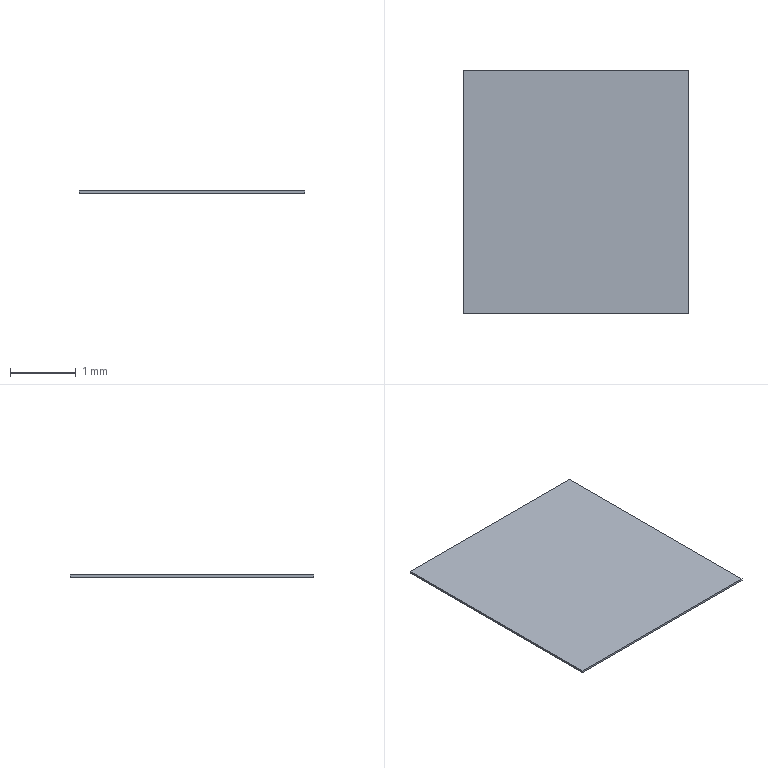Part | Creo | 1 solid | 6 faces | box 3.43 x 3.71 x 0.03048 mm | volume 0.3879 mm3 | plane 6
STEP:
#1=CARTESIAN_POINT('',(0.,0.,0.));
#2=DIRECTION('',(0.,0.,1.));
#3=DIRECTION('',(1.,0.,0.));
#4=AXIS2_PLACEMENT_3D('',#1,#2,#3);
#5=CARTESIAN_POINT('',(-1.775,-1.855,0.));
#6=VERTEX_POINT('',#5);
#7=CARTESIAN_POINT('',(1.655,-1.855,0.));
#8=VERTEX_POINT('',#7);
#9=CARTESIAN_POINT('',(-1.775,-1.855,0.));
#10=DIRECTION('',(1.,0.,0.));
#11=VECTOR('',#10,3.43);
#12=LINE('',#9,#11);
#13=EDGE_CURVE('',#6,#8,#12,.T.);
#14=ORIENTED_EDGE('',*,*,#13,.T.);
#15=CARTESIAN_POINT('',(1.655,1.855,0.));
#16=VERTEX_POINT('',#15);
#17=CARTESIAN_POINT('',(1.655,-1.855,0.));
#18=DIRECTION('',(0.,1.,0.));
#19=VECTOR('',#18,3.71);
#20=LINE('',#17,#19);
#21=EDGE_CURVE('',#8,#16,#20,.T.);
#22=ORIENTED_EDGE('',*,*,#21,.T.);
#23=CARTESIAN_POINT('',(-1.775,1.855,0.));
#24=VERTEX_POINT('',#23);
#25=CARTESIAN_POINT('',(1.655,1.855,0.));
#26=DIRECTION('',(-1.,0.,0.));
#27=VECTOR('',#26,3.43);
#28=LINE('',#25,#27);
#29=EDGE_CURVE('',#16,#24,#28,.T.);
#30=ORIENTED_EDGE('',*,*,#29,.T.);
#31=CARTESIAN_POINT('',(-1.775,1.855,0.));
#32=DIRECTION('',(0.,-1.,0.));
#33=VECTOR('',#32,3.71);
#34=LINE('',#31,#33);
#35=EDGE_CURVE('',#24,#6,#34,.T.);
#36=ORIENTED_EDGE('',*,*,#35,.T.);
#37=EDGE_LOOP('',(#14,#22,#30,#36));
#38=FACE_OUTER_BOUND('',#37,.F.);
#39=CARTESIAN_POINT('',(0.,0.,0.));
#40=DIRECTION('',(0.,0.,1.));
#41=DIRECTION('',(1.,0.,0.));
#42=AXIS2_PLACEMENT_3D('',#39,#40,#41);
#43=PLANE('',#42);
#44=ADVANCED_FACE('',(#38),#43,.F.);
#45=ORIENTED_EDGE('',*,*,#13,.F.);
#46=CARTESIAN_POINT('',(-1.775,-1.855,0.03048));
#47=VERTEX_POINT('',#46);
#48=CARTESIAN_POINT('',(-1.775,-1.855,0.));
#49=DIRECTION('',(0.,0.,1.));
#50=VECTOR('',#49,0.03048);
#51=LINE('',#48,#50);
#52=EDGE_CURVE('',#6,#47,#51,.T.);
#53=ORIENTED_EDGE('',*,*,#52,.T.);
#54=CARTESIAN_POINT('',(1.655,-1.855,0.03048));
#55=VERTEX_POINT('',#54);
#56=CARTESIAN_POINT('',(-1.775,-1.855,0.03048));
#57=DIRECTION('',(1.,0.,0.));
#58=VECTOR('',#57,3.43);
#59=LINE('',#56,#58);
#60=EDGE_CURVE('',#47,#55,#59,.T.);
#61=ORIENTED_EDGE('',*,*,#60,.T.);
#62=CARTESIAN_POINT('',(1.655,-1.855,0.));
#63=DIRECTION('',(0.,0.,1.));
#64=VECTOR('',#63,0.03048);
#65=LINE('',#62,#64);
#66=EDGE_CURVE('',#8,#55,#65,.T.);
#67=ORIENTED_EDGE('',*,*,#66,.F.);
#68=EDGE_LOOP('',(#45,#53,#61,#67));
#69=FACE_OUTER_BOUND('',#68,.F.);
#70=CARTESIAN_POINT('',(-1.775,-1.855,0.));
#71=DIRECTION('',(0.,-1.,0.));
#72=DIRECTION('',(1.,0.,0.));
#73=AXIS2_PLACEMENT_3D('',#70,#71,#72);
#74=PLANE('',#73);
#75=ADVANCED_FACE('',(#69),#74,.T.);
#76=ORIENTED_EDGE('',*,*,#35,.F.);
#77=CARTESIAN_POINT('',(-1.775,1.855,0.03048));
#78=VERTEX_POINT('',#77);
#79=CARTESIAN_POINT('',(-1.775,1.855,0.));
#80=DIRECTION('',(0.,0.,1.));
#81=VECTOR('',#80,0.03048);
#82=LINE('',#79,#81);
#83=EDGE_CURVE('',#24,#78,#82,.T.);
#84=ORIENTED_EDGE('',*,*,#83,.T.);
#85=CARTESIAN_POINT('',(-1.775,1.855,0.03048));
#86=DIRECTION('',(0.,-1.,0.));
#87=VECTOR('',#86,3.71);
#88=LINE('',#85,#87);
#89=EDGE_CURVE('',#78,#47,#88,.T.);
#90=ORIENTED_EDGE('',*,*,#89,.T.);
#91=ORIENTED_EDGE('',*,*,#52,.F.);
#92=EDGE_LOOP('',(#76,#84,#90,#91));
#93=FACE_OUTER_BOUND('',#92,.F.);
#94=CARTESIAN_POINT('',(-1.775,1.855,0.));
#95=DIRECTION('',(-1.,0.,0.));
#96=DIRECTION('',(0.,-1.,0.));
#97=AXIS2_PLACEMENT_3D('',#94,#95,#96);
#98=PLANE('',#97);
#99=ADVANCED_FACE('',(#93),#98,.T.);
#100=ORIENTED_EDGE('',*,*,#29,.F.);
#101=CARTESIAN_POINT('',(1.655,1.855,0.03048));
#102=VERTEX_POINT('',#101);
#103=CARTESIAN_POINT('',(1.655,1.855,0.));
#104=DIRECTION('',(0.,0.,1.));
#105=VECTOR('',#104,0.03048);
#106=LINE('',#103,#105);
#107=EDGE_CURVE('',#16,#102,#106,.T.);
#108=ORIENTED_EDGE('',*,*,#107,.T.);
#109=CARTESIAN_POINT('',(1.655,1.855,0.03048));
#110=DIRECTION('',(-1.,0.,0.));
#111=VECTOR('',#110,3.43);
#112=LINE('',#109,#111);
#113=EDGE_CURVE('',#102,#78,#112,.T.);
#114=ORIENTED_EDGE('',*,*,#113,.T.);
#115=ORIENTED_EDGE('',*,*,#83,.F.);
#116=EDGE_LOOP('',(#100,#108,#114,#115));
#117=FACE_OUTER_BOUND('',#116,.F.);
#118=CARTESIAN_POINT('',(1.655,1.855,0.));
#119=DIRECTION('',(0.,1.,0.));
#120=DIRECTION('',(-1.,0.,0.));
#121=AXIS2_PLACEMENT_3D('',#118,#119,#120);
#122=PLANE('',#121);
#123=ADVANCED_FACE('',(#117),#122,.T.);
#124=ORIENTED_EDGE('',*,*,#21,.F.);
#125=ORIENTED_EDGE('',*,*,#66,.T.);
#126=CARTESIAN_POINT('',(1.655,-1.855,0.03048));
#127=DIRECTION('',(0.,1.,0.));
#128=VECTOR('',#127,3.71);
#129=LINE('',#126,#128);
#130=EDGE_CURVE('',#55,#102,#129,.T.);
#131=ORIENTED_EDGE('',*,*,#130,.T.);
#132=ORIENTED_EDGE('',*,*,#107,.F.);
#133=EDGE_LOOP('',(#124,#125,#131,#132));
#134=FACE_OUTER_BOUND('',#133,.F.);
#135=CARTESIAN_POINT('',(1.655,-1.855,0.));
#136=DIRECTION('',(1.,0.,0.));
#137=DIRECTION('',(0.,1.,0.));
#138=AXIS2_PLACEMENT_3D('',#135,#136,#137);
#139=PLANE('',#138);
#140=ADVANCED_FACE('',(#134),#139,.T.);
#141=ORIENTED_EDGE('',*,*,#60,.F.);
#142=ORIENTED_EDGE('',*,*,#89,.F.);
#143=ORIENTED_EDGE('',*,*,#113,.F.);
#144=ORIENTED_EDGE('',*,*,#130,.F.);
#145=EDGE_LOOP('',(#141,#142,#143,#144));
#146=FACE_OUTER_BOUND('',#145,.F.);
#147=CARTESIAN_POINT('',(0.,0.,0.03048));
#148=DIRECTION('',(0.,0.,1.));
#149=DIRECTION('',(1.,0.,0.));
#150=AXIS2_PLACEMENT_3D('',#147,#148,#149);
#151=PLANE('',#150);
#152=ADVANCED_FACE('',(#146),#151,.T.);
#153=CLOSED_SHELL('',(#44,#75,#99,#123,#140,#152));
#154=MANIFOLD_SOLID_BREP('',#153);
#155=(LENGTH_UNIT()NAMED_UNIT(*)SI_UNIT(.MILLI.,.METRE.));
#156=UNCERTAINTY_MEASURE_WITH_UNIT(LENGTH_MEASURE(0.0005053),#155,'','');
#157=(NAMED_UNIT(*)PLANE_ANGLE_UNIT()SI_UNIT($,.RADIAN.));
#158=PLANE_ANGLE_MEASURE_WITH_UNIT(PLANE_ANGLE_MEASURE(0.01745),#157);
#159=(CONVERSION_BASED_UNIT('DEGREE',#158)NAMED_UNIT(*)PLANE_ANGLE_UNIT());
#160=(NAMED_UNIT(*)SI_UNIT($,.STERADIAN.)SOLID_ANGLE_UNIT());
#161=(GEOMETRIC_REPRESENTATION_CONTEXT(3)GLOBAL_UNCERTAINTY_ASSIGNED_CONTEXT((#156))GLOBAL_UNIT_ASSIGNED_CONTEXT((#155,#159,#160))REPRESENTATION_CONTEXT('',''));
#162=ADVANCED_BREP_SHAPE_REPRESENTATION('',(#4,#154),#161);